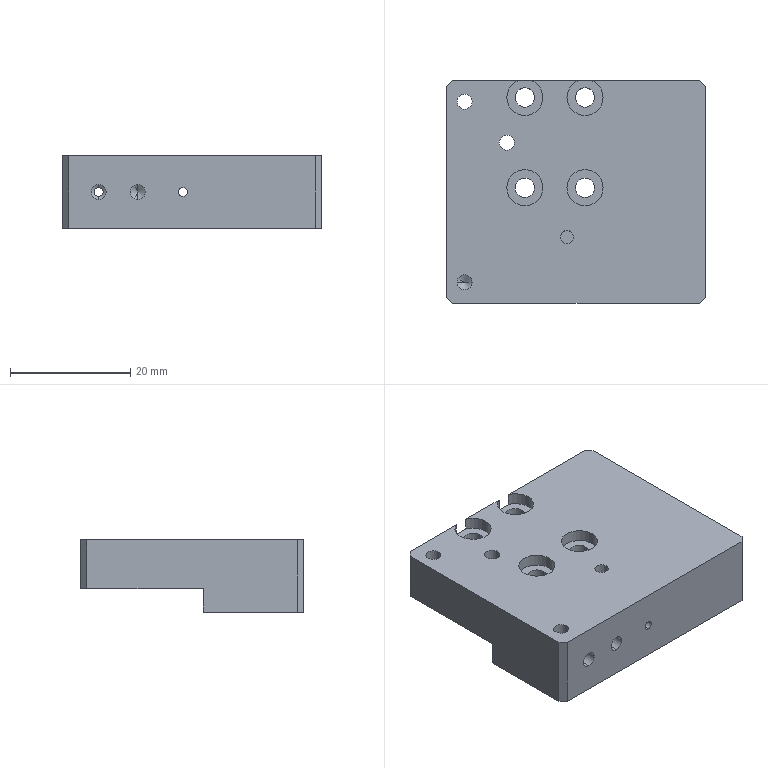Part | SolidWorks | features HoleWzd 6, ICE 4, MoveFace 2, Chamfer 1, Extrusion 1, LPattern 1, RefAxis 1 | 1 solid | 71 faces | box 43 x 37 x 12 mm | volume 14568 mm3 | cylinder 42 | plane 17 | cone 12 | commonest cylinder face diameters 2.5 x10 6 x10 3.2 x8 1.5 x6 3.3 x6 2.2 x2